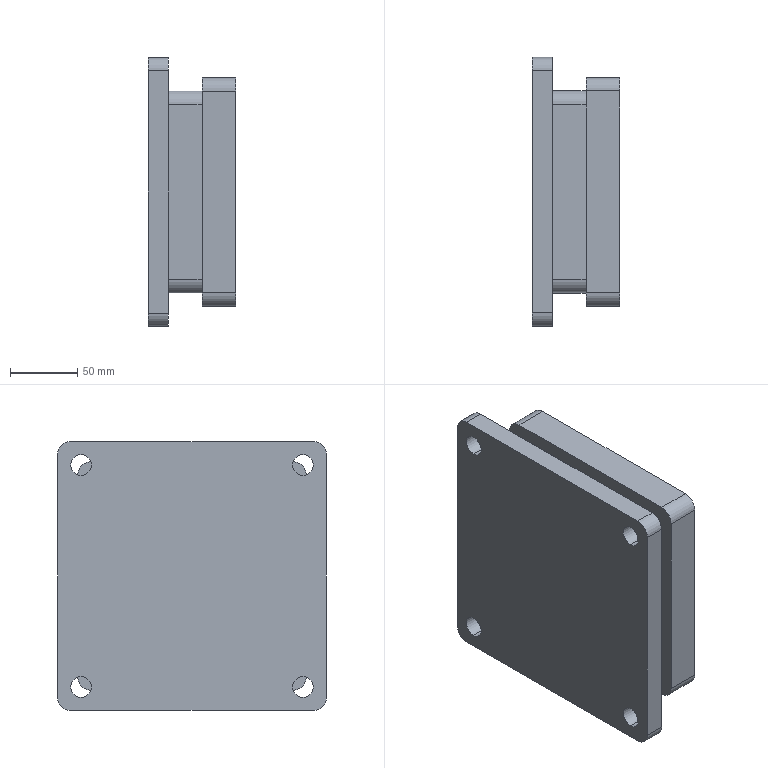Part | STEP file | part 322(default_machined_)-1.STEP | 2 solids | 46 faces | box 65 x 200 x 200 mm | volume 1280743 mm3 | cylinder 24 | plane 22 | commonest cylinder face diameters 20 x12 15.5 x8 10 x4
STEP:
#1=CARTESIAN_POINT('',(30.,-75.,85.));
#2=VERTEX_POINT('',#1);
#3=CARTESIAN_POINT('',(5.,-75.,85.));
#4=VERTEX_POINT('',#3);
#5=CARTESIAN_POINT('',(30.,-75.,85.));
#6=DIRECTION('',(-1.,0.,0.));
#7=VECTOR('',#6,1000.);
#8=LINE('',#5,#7);
#9=EDGE_CURVE('',#2,#4,#8,.T.);
#10=ORIENTED_EDGE('',*,*,#9,.T.);
#11=CARTESIAN_POINT('',(5.,-85.,75.));
#12=VERTEX_POINT('',#11);
#13=CARTESIAN_POINT('',(5.,-75.,75.));
#14=DIRECTION('',(1.,0.,0.));
#15=DIRECTION('',(0.,0.,-1.));
#16=AXIS2_PLACEMENT_3D('',#13,#14,#15);
#17=CIRCLE('',#16,10.);
#18=EDGE_CURVE('',#4,#12,#17,.T.);
#19=ORIENTED_EDGE('',*,*,#18,.T.);
#20=CARTESIAN_POINT('',(30.,-85.,75.));
#21=VERTEX_POINT('',#20);
#22=CARTESIAN_POINT('',(30.,-85.,75.));
#23=DIRECTION('',(-1.,0.,0.));
#24=VECTOR('',#23,1000.);
#25=LINE('',#22,#24);
#26=EDGE_CURVE('',#21,#12,#25,.T.);
#27=ORIENTED_EDGE('',*,*,#26,.F.);
#28=CARTESIAN_POINT('',(30.,-75.,75.));
#29=DIRECTION('',(1.,0.,0.));
#30=DIRECTION('',(0.,0.,-1.));
#31=AXIS2_PLACEMENT_3D('',#28,#29,#30);
#32=CIRCLE('',#31,10.);
#33=EDGE_CURVE('',#2,#21,#32,.T.);
#34=ORIENTED_EDGE('',*,*,#33,.F.);
#35=EDGE_LOOP('',(#10,#19,#27,#34));
#36=FACE_OUTER_BOUND('',#35,.T.);
#37=CARTESIAN_POINT('',(30.,-75.,75.));
#38=DIRECTION('',(-1.,0.,0.));
#39=DIRECTION('',(0.,0.,1.));
#40=AXIS2_PLACEMENT_3D('',#37,#38,#39);
#41=CYLINDRICAL_SURFACE('',#40,10.);
#42=ADVANCED_FACE('',(#36),#41,.T.);
#43=CARTESIAN_POINT('',(30.,75.,85.));
#44=VERTEX_POINT('',#43);
#45=CARTESIAN_POINT('',(5.,75.,85.));
#46=VERTEX_POINT('',#45);
#47=CARTESIAN_POINT('',(30.,75.,85.));
#48=DIRECTION('',(-1.,0.,0.));
#49=VECTOR('',#48,1000.);
#50=LINE('',#47,#49);
#51=EDGE_CURVE('',#44,#46,#50,.T.);
#52=ORIENTED_EDGE('',*,*,#51,.T.);
#53=CARTESIAN_POINT('',(5.,75.,85.));
#54=DIRECTION('',(0.,-1.,0.));
#55=VECTOR('',#54,1000.);
#56=LINE('',#53,#55);
#57=EDGE_CURVE('',#46,#4,#56,.T.);
#58=ORIENTED_EDGE('',*,*,#57,.T.);
#59=ORIENTED_EDGE('',*,*,#9,.F.);
#60=CARTESIAN_POINT('',(30.,75.,85.));
#61=DIRECTION('',(0.,-1.,0.));
#62=VECTOR('',#61,1000.);
#63=LINE('',#60,#62);
#64=EDGE_CURVE('',#44,#2,#63,.T.);
#65=ORIENTED_EDGE('',*,*,#64,.F.);
#66=EDGE_LOOP('',(#52,#58,#59,#65));
#67=FACE_OUTER_BOUND('',#66,.T.);
#68=CARTESIAN_POINT('',(30.,75.,85.));
#69=DIRECTION('',(0.,0.,-1.));
#70=DIRECTION('',(-1.,0.,0.));
#71=AXIS2_PLACEMENT_3D('',#68,#69,#70);
#72=PLANE('',#71);
#73=ADVANCED_FACE('',(#67),#72,.F.);
#74=CARTESIAN_POINT('',(30.,85.,75.));
#75=VERTEX_POINT('',#74);
#76=CARTESIAN_POINT('',(5.,85.,75.));
#77=VERTEX_POINT('',#76);
#78=CARTESIAN_POINT('',(30.,85.,75.));
#79=DIRECTION('',(-1.,0.,0.));
#80=VECTOR('',#79,1000.);
#81=LINE('',#78,#80);
#82=EDGE_CURVE('',#75,#77,#81,.T.);
#83=ORIENTED_EDGE('',*,*,#82,.T.);
#84=CARTESIAN_POINT('',(5.,75.,75.));
#85=DIRECTION('',(1.,0.,0.));
#86=DIRECTION('',(0.,0.,-1.));
#87=AXIS2_PLACEMENT_3D('',#84,#85,#86);
#88=CIRCLE('',#87,10.);
#89=EDGE_CURVE('',#77,#46,#88,.T.);
#90=ORIENTED_EDGE('',*,*,#89,.T.);
#91=ORIENTED_EDGE('',*,*,#51,.F.);
#92=CARTESIAN_POINT('',(30.,75.,75.));
#93=DIRECTION('',(1.,0.,0.));
#94=DIRECTION('',(0.,0.,-1.));
#95=AXIS2_PLACEMENT_3D('',#92,#93,#94);
#96=CIRCLE('',#95,10.);
#97=EDGE_CURVE('',#75,#44,#96,.T.);
#98=ORIENTED_EDGE('',*,*,#97,.F.);
#99=EDGE_LOOP('',(#83,#90,#91,#98));
#100=FACE_OUTER_BOUND('',#99,.T.);
#101=CARTESIAN_POINT('',(30.,75.,75.));
#102=DIRECTION('',(-1.,0.,0.));
#103=DIRECTION('',(0.,0.,1.));
#104=AXIS2_PLACEMENT_3D('',#101,#102,#103);
#105=CYLINDRICAL_SURFACE('',#104,10.);
#106=ADVANCED_FACE('',(#100),#105,.T.);
#107=CARTESIAN_POINT('',(30.,85.,-75.));
#108=VERTEX_POINT('',#107);
#109=CARTESIAN_POINT('',(5.,85.,-75.));
#110=VERTEX_POINT('',#109);
#111=CARTESIAN_POINT('',(30.,85.,-75.));
#112=DIRECTION('',(-1.,0.,0.));
#113=VECTOR('',#112,1000.);
#114=LINE('',#111,#113);
#115=EDGE_CURVE('',#108,#110,#114,.T.);
#116=ORIENTED_EDGE('',*,*,#115,.T.);
#117=CARTESIAN_POINT('',(5.,85.,75.));
#118=DIRECTION('',(0.,0.,1.));
#119=VECTOR('',#118,1000.);
#120=LINE('',#117,#119);
#121=EDGE_CURVE('',#110,#77,#120,.T.);
#122=ORIENTED_EDGE('',*,*,#121,.T.);
#123=ORIENTED_EDGE('',*,*,#82,.F.);
#124=CARTESIAN_POINT('',(30.,85.,-75.));
#125=DIRECTION('',(0.,0.,1.));
#126=VECTOR('',#125,1000.);
#127=LINE('',#124,#126);
#128=EDGE_CURVE('',#108,#75,#127,.T.);
#129=ORIENTED_EDGE('',*,*,#128,.F.);
#130=EDGE_LOOP('',(#116,#122,#123,#129));
#131=FACE_OUTER_BOUND('',#130,.T.);
#132=CARTESIAN_POINT('',(30.,85.,-75.));
#133=DIRECTION('',(0.,-1.,0.));
#134=DIRECTION('',(0.,0.,-1.));
#135=AXIS2_PLACEMENT_3D('',#132,#133,#134);
#136=PLANE('',#135);
#137=ADVANCED_FACE('',(#131),#136,.F.);
#138=CARTESIAN_POINT('',(30.,75.,-85.));
#139=VERTEX_POINT('',#138);
#140=CARTESIAN_POINT('',(5.,75.,-85.));
#141=VERTEX_POINT('',#140);
#142=CARTESIAN_POINT('',(30.,75.,-85.));
#143=DIRECTION('',(-1.,0.,0.));
#144=VECTOR('',#143,1000.);
#145=LINE('',#142,#144);
#146=EDGE_CURVE('',#139,#141,#145,.T.);
#147=ORIENTED_EDGE('',*,*,#146,.T.);
#148=CARTESIAN_POINT('',(5.,75.,-75.));
#149=DIRECTION('',(1.,0.,0.));
#150=DIRECTION('',(0.,0.,-1.));
#151=AXIS2_PLACEMENT_3D('',#148,#149,#150);
#152=CIRCLE('',#151,10.);
#153=EDGE_CURVE('',#141,#110,#152,.T.);
#154=ORIENTED_EDGE('',*,*,#153,.T.);
#155=ORIENTED_EDGE('',*,*,#115,.F.);
#156=CARTESIAN_POINT('',(30.,75.,-75.));
#157=DIRECTION('',(1.,0.,0.));
#158=DIRECTION('',(0.,0.,-1.));
#159=AXIS2_PLACEMENT_3D('',#156,#157,#158);
#160=CIRCLE('',#159,10.);
#161=EDGE_CURVE('',#139,#108,#160,.T.);
#162=ORIENTED_EDGE('',*,*,#161,.F.);
#163=EDGE_LOOP('',(#147,#154,#155,#162));
#164=FACE_OUTER_BOUND('',#163,.T.);
#165=CARTESIAN_POINT('',(30.,75.,-75.));
#166=DIRECTION('',(-1.,0.,0.));
#167=DIRECTION('',(0.,0.,1.));
#168=AXIS2_PLACEMENT_3D('',#165,#166,#167);
#169=CYLINDRICAL_SURFACE('',#168,10.);
#170=ADVANCED_FACE('',(#164),#169,.T.);
#171=CARTESIAN_POINT('',(30.,-75.,-85.));
#172=VERTEX_POINT('',#171);
#173=CARTESIAN_POINT('',(5.,-75.,-85.));
#174=VERTEX_POINT('',#173);
#175=CARTESIAN_POINT('',(30.,-75.,-85.));
#176=DIRECTION('',(-1.,0.,0.));
#177=VECTOR('',#176,1000.);
#178=LINE('',#175,#177);
#179=EDGE_CURVE('',#172,#174,#178,.T.);
#180=ORIENTED_EDGE('',*,*,#179,.T.);
#181=CARTESIAN_POINT('',(5.,75.,-85.));
#182=DIRECTION('',(0.,1.,0.));
#183=VECTOR('',#182,1000.);
#184=LINE('',#181,#183);
#185=EDGE_CURVE('',#174,#141,#184,.T.);
#186=ORIENTED_EDGE('',*,*,#185,.T.);
#187=ORIENTED_EDGE('',*,*,#146,.F.);
#188=CARTESIAN_POINT('',(30.,-75.,-85.));
#189=DIRECTION('',(0.,1.,0.));
#190=VECTOR('',#189,1000.);
#191=LINE('',#188,#190);
#192=EDGE_CURVE('',#172,#139,#191,.T.);
#193=ORIENTED_EDGE('',*,*,#192,.F.);
#194=EDGE_LOOP('',(#180,#186,#187,#193));
#195=FACE_OUTER_BOUND('',#194,.T.);
#196=CARTESIAN_POINT('',(30.,-75.,-85.));
#197=DIRECTION('',(0.,0.,1.));
#198=DIRECTION('',(0.,-1.,0.));
#199=AXIS2_PLACEMENT_3D('',#196,#197,#198);
#200=PLANE('',#199);
#201=ADVANCED_FACE('',(#195),#200,.F.);
#202=CARTESIAN_POINT('',(30.,-85.,-75.));
#203=VERTEX_POINT('',#202);
#204=CARTESIAN_POINT('',(5.,-85.,-75.));
#205=VERTEX_POINT('',#204);
#206=CARTESIAN_POINT('',(30.,-85.,-75.));
#207=DIRECTION('',(-1.,0.,0.));
#208=VECTOR('',#207,1000.);
#209=LINE('',#206,#208);
#210=EDGE_CURVE('',#203,#205,#209,.T.);
#211=ORIENTED_EDGE('',*,*,#210,.T.);
#212=CARTESIAN_POINT('',(5.,-75.,-75.));
#213=DIRECTION('',(1.,0.,0.));
#214=DIRECTION('',(0.,0.,-1.));
#215=AXIS2_PLACEMENT_3D('',#212,#213,#214);
#216=CIRCLE('',#215,10.);
#217=EDGE_CURVE('',#205,#174,#216,.T.);
#218=ORIENTED_EDGE('',*,*,#217,.T.);
#219=ORIENTED_EDGE('',*,*,#179,.F.);
#220=CARTESIAN_POINT('',(30.,-75.,-75.));
#221=DIRECTION('',(1.,0.,0.));
#222=DIRECTION('',(0.,0.,-1.));
#223=AXIS2_PLACEMENT_3D('',#220,#221,#222);
#224=CIRCLE('',#223,10.);
#225=EDGE_CURVE('',#203,#172,#224,.T.);
#226=ORIENTED_EDGE('',*,*,#225,.F.);
#227=EDGE_LOOP('',(#211,#218,#219,#226));
#228=FACE_OUTER_BOUND('',#227,.T.);
#229=CARTESIAN_POINT('',(30.,-75.,-75.));
#230=DIRECTION('',(-1.,0.,0.));
#231=DIRECTION('',(0.,0.,1.));
#232=AXIS2_PLACEMENT_3D('',#229,#230,#231);
#233=CYLINDRICAL_SURFACE('',#232,10.);
#234=ADVANCED_FACE('',(#228),#233,.T.);
#235=ORIENTED_EDGE('',*,*,#26,.T.);
#236=CARTESIAN_POINT('',(5.,-85.,75.));
#237=DIRECTION('',(0.,0.,-1.));
#238=VECTOR('',#237,1000.);
#239=LINE('',#236,#238);
#240=EDGE_CURVE('',#12,#205,#239,.T.);
#241=ORIENTED_EDGE('',*,*,#240,.T.);
#242=ORIENTED_EDGE('',*,*,#210,.F.);
#243=CARTESIAN_POINT('',(30.,-85.,75.));
#244=DIRECTION('',(0.,0.,-1.));
#245=VECTOR('',#244,1000.);
#246=LINE('',#243,#245);
#247=EDGE_CURVE('',#21,#203,#246,.T.);
#248=ORIENTED_EDGE('',*,*,#247,.F.);
#249=EDGE_LOOP('',(#235,#241,#242,#248));
#250=FACE_OUTER_BOUND('',#249,.T.);
#251=CARTESIAN_POINT('',(30.,-85.,75.));
#252=DIRECTION('',(0.,1.,0.));
#253=DIRECTION('',(0.,0.,-1.));
#254=AXIS2_PLACEMENT_3D('',#251,#252,#253);
#255=PLANE('',#254);
#256=ADVANCED_FACE('',(#250),#255,.F.);
#257=ORIENTED_EDGE('',*,*,#33,.T.);
#258=ORIENTED_EDGE('',*,*,#247,.T.);
#259=ORIENTED_EDGE('',*,*,#225,.T.);
#260=ORIENTED_EDGE('',*,*,#192,.T.);
#261=ORIENTED_EDGE('',*,*,#161,.T.);
#262=ORIENTED_EDGE('',*,*,#128,.T.);
#263=ORIENTED_EDGE('',*,*,#97,.T.);
#264=ORIENTED_EDGE('',*,*,#64,.T.);
#265=EDGE_LOOP('',(#257,#258,#259,#260,#261,#262,#263,#264));
#266=FACE_OUTER_BOUND('',#265,.T.);
#267=CARTESIAN_POINT('',(30.,-75.,75.));
#268=DIRECTION('',(1.,0.,0.));
#269=DIRECTION('',(0.,1.,0.));
#270=AXIS2_PLACEMENT_3D('',#267,#268,#269);
#271=PLANE('',#270);
#272=ADVANCED_FACE('',(#266),#271,.T.);
#273=CARTESIAN_POINT('',(5.,75.,-65.));
#274=VERTEX_POINT('',#273);
#275=CARTESIAN_POINT('',(5.,75.,65.));
#276=VERTEX_POINT('',#275);
#277=CARTESIAN_POINT('',(5.,75.,-65.));
#278=DIRECTION('',(0.,0.,1.));
#279=VECTOR('',#278,1000.);
#280=LINE('',#277,#279);
#281=EDGE_CURVE('',#274,#276,#280,.T.);
#282=ORIENTED_EDGE('',*,*,#281,.T.);
#283=CARTESIAN_POINT('',(5.,65.,75.));
#284=VERTEX_POINT('',#283);
#285=CARTESIAN_POINT('',(5.,65.,65.));
#286=DIRECTION('',(1.,0.,0.));
#287=DIRECTION('',(0.,0.,-1.));
#288=AXIS2_PLACEMENT_3D('',#285,#286,#287);
#289=CIRCLE('',#288,10.);
#290=EDGE_CURVE('',#276,#284,#289,.T.);
#291=ORIENTED_EDGE('',*,*,#290,.T.);
#292=CARTESIAN_POINT('',(5.,-65.,75.));
#293=VERTEX_POINT('',#292);
#294=CARTESIAN_POINT('',(5.,65.,75.));
#295=DIRECTION('',(0.,-1.,0.));
#296=VECTOR('',#295,1000.);
#297=LINE('',#294,#296);
#298=EDGE_CURVE('',#284,#293,#297,.T.);
#299=ORIENTED_EDGE('',*,*,#298,.T.);
#300=CARTESIAN_POINT('',(5.,-75.,65.));
#301=VERTEX_POINT('',#300);
#302=CARTESIAN_POINT('',(5.,-65.,65.));
#303=DIRECTION('',(1.,0.,0.));
#304=DIRECTION('',(0.,0.,-1.));
#305=AXIS2_PLACEMENT_3D('',#302,#303,#304);
#306=CIRCLE('',#305,10.);
#307=EDGE_CURVE('',#293,#301,#306,.T.);
#308=ORIENTED_EDGE('',*,*,#307,.T.);
#309=CARTESIAN_POINT('',(5.,-75.,-65.));
#310=VERTEX_POINT('',#309);
#311=CARTESIAN_POINT('',(5.,-75.,65.));
#312=DIRECTION('',(0.,0.,-1.));
#313=VECTOR('',#312,1000.);
#314=LINE('',#311,#313);
#315=EDGE_CURVE('',#301,#310,#314,.T.);
#316=ORIENTED_EDGE('',*,*,#315,.T.);
#317=CARTESIAN_POINT('',(5.,-65.,-75.));
#318=VERTEX_POINT('',#317);
#319=CARTESIAN_POINT('',(5.,-65.,-65.));
#320=DIRECTION('',(1.,0.,0.));
#321=DIRECTION('',(0.,0.,-1.));
#322=AXIS2_PLACEMENT_3D('',#319,#320,#321);
#323=CIRCLE('',#322,10.);
#324=EDGE_CURVE('',#310,#318,#323,.T.);
#325=ORIENTED_EDGE('',*,*,#324,.T.);
#326=CARTESIAN_POINT('',(5.,65.,-75.));
#327=VERTEX_POINT('',#326);
#328=CARTESIAN_POINT('',(5.,-65.,-75.));
#329=DIRECTION('',(0.,1.,0.));
#330=VECTOR('',#329,1000.);
#331=LINE('',#328,#330);
#332=EDGE_CURVE('',#318,#327,#331,.T.);
#333=ORIENTED_EDGE('',*,*,#332,.T.);
#334=CARTESIAN_POINT('',(5.,65.,-65.));
#335=DIRECTION('',(1.,0.,0.));
#336=DIRECTION('',(0.,0.,-1.));
#337=AXIS2_PLACEMENT_3D('',#334,#335,#336);
#338=CIRCLE('',#337,10.);
#339=EDGE_CURVE('',#327,#274,#338,.T.);
#340=ORIENTED_EDGE('',*,*,#339,.T.);
#341=EDGE_LOOP('',(#282,#291,#299,#308,#316,#325,#333,#340));
#342=FACE_BOUND('',#341,.T.);
#343=ORIENTED_EDGE('',*,*,#18,.F.);
#344=ORIENTED_EDGE('',*,*,#57,.F.);
#345=ORIENTED_EDGE('',*,*,#89,.F.);
#346=ORIENTED_EDGE('',*,*,#121,.F.);
#347=ORIENTED_EDGE('',*,*,#153,.F.);
#348=ORIENTED_EDGE('',*,*,#185,.F.);
#349=ORIENTED_EDGE('',*,*,#217,.F.);
#350=ORIENTED_EDGE('',*,*,#240,.F.);
#351=EDGE_LOOP('',(#343,#344,#345,#346,#347,#348,#349,#350));
#352=FACE_OUTER_BOUND('',#351,.T.);
#353=CARTESIAN_POINT('',(5.,-75.,75.));
#354=DIRECTION('',(1.,0.,0.));
#355=DIRECTION('',(0.,1.,0.));
#356=AXIS2_PLACEMENT_3D('',#353,#354,#355);
#357=PLANE('',#356);
#358=ADVANCED_FACE('',(#342,#352),#357,.F.);
#359=CARTESIAN_POINT('',(10.,65.,-70.));
#360=VERTEX_POINT('',#359);
#361=CARTESIAN_POINT('',(10.,70.,-65.));
#362=VERTEX_POINT('',#361);
#363=CARTESIAN_POINT('',(10.,65.,-65.));
#364=DIRECTION('',(1.,0.,0.));
#365=DIRECTION('',(0.,0.,-1.));
#366=AXIS2_PLACEMENT_3D('',#363,#364,#365);
#367=CIRCLE('',#366,5.);
#368=EDGE_CURVE('',#360,#362,#367,.T.);
#369=ORIENTED_EDGE('',*,*,#368,.F.);
#370=CARTESIAN_POINT('',(10.,-65.,-70.));
#371=VERTEX_POINT('',#370);
#372=CARTESIAN_POINT('',(10.,-65.,-70.));
#373=DIRECTION('',(0.,1.,0.));
#374=VECTOR('',#373,1000.);
#375=LINE('',#372,#374);
#376=EDGE_CURVE('',#371,#360,#375,.T.);
#377=ORIENTED_EDGE('',*,*,#376,.F.);
#378=CARTESIAN_POINT('',(10.,-70.,-65.));
#379=VERTEX_POINT('',#378);
#380=CARTESIAN_POINT('',(10.,-65.,-65.));
#381=DIRECTION('',(1.,0.,0.));
#382=DIRECTION('',(0.,0.,-1.));
#383=AXIS2_PLACEMENT_3D('',#380,#381,#382);
#384=CIRCLE('',#383,5.);
#385=EDGE_CURVE('',#379,#371,#384,.T.);
#386=ORIENTED_EDGE('',*,*,#385,.F.);
#387=CARTESIAN_POINT('',(10.,-70.,65.));
#388=VERTEX_POINT('',#387);
#389=CARTESIAN_POINT('',(10.,-70.,65.));
#390=DIRECTION('',(0.,0.,-1.));
#391=VECTOR('',#390,1000.);
#392=LINE('',#389,#391);
#393=EDGE_CURVE('',#388,#379,#392,.T.);
#394=ORIENTED_EDGE('',*,*,#393,.F.);
#395=CARTESIAN_POINT('',(10.,-65.,70.));
#396=VERTEX_POINT('',#395);
#397=CARTESIAN_POINT('',(10.,-65.,65.));
#398=DIRECTION('',(1.,0.,0.));
#399=DIRECTION('',(0.,0.,-1.));
#400=AXIS2_PLACEMENT_3D('',#397,#398,#399);
#401=CIRCLE('',#400,5.);
#402=EDGE_CURVE('',#396,#388,#401,.T.);
#403=ORIENTED_EDGE('',*,*,#402,.F.);
#404=CARTESIAN_POINT('',(10.,65.,70.));
#405=VERTEX_POINT('',#404);
#406=CARTESIAN_POINT('',(10.,65.,70.));
#407=DIRECTION('',(0.,-1.,0.));
#408=VECTOR('',#407,1000.);
#409=LINE('',#406,#408);
#410=EDGE_CURVE('',#405,#396,#409,.T.);
#411=ORIENTED_EDGE('',*,*,#410,.F.);
#412=CARTESIAN_POINT('',(10.,70.,65.));
#413=VERTEX_POINT('',#412);
#414=CARTESIAN_POINT('',(10.,65.,65.));
#415=DIRECTION('',(1.,0.,0.));
#416=DIRECTION('',(0.,0.,-1.));
#417=AXIS2_PLACEMENT_3D('',#414,#415,#416);
#418=CIRCLE('',#417,5.);
#419=EDGE_CURVE('',#413,#405,#418,.T.);
#420=ORIENTED_EDGE('',*,*,#419,.F.);
#421=CARTESIAN_POINT('',(10.,70.,-65.));
#422=DIRECTION('',(0.,0.,1.));
#423=VECTOR('',#422,1000.);
#424=LINE('',#421,#423);
#425=EDGE_CURVE('',#362,#413,#424,.T.);
#426=ORIENTED_EDGE('',*,*,#425,.F.);
#427=EDGE_LOOP('',(#369,#377,#386,#394,#403,#411,#420,#426));
#428=FACE_OUTER_BOUND('',#427,.T.);
#429=CARTESIAN_POINT('',(10.,65.,-65.));
#430=DIRECTION('',(1.,0.,0.));
#431=DIRECTION('',(0.,1.,0.));
#432=AXIS2_PLACEMENT_3D('',#429,#430,#431);
#433=PLANE('',#432);
#434=ADVANCED_FACE('',(#428),#433,.F.);
#435=CARTESIAN_POINT('',(-20.,-65.,70.));
#436=VERTEX_POINT('',#435);
#437=CARTESIAN_POINT('',(-20.,-70.,65.));
#438=VERTEX_POINT('',#437);
#439=CARTESIAN_POINT('',(-20.,-65.,65.));
#440=DIRECTION('',(1.,0.,0.));
#441=DIRECTION('',(0.,1.,0.));
#442=AXIS2_PLACEMENT_3D('',#439,#440,#441);
#443=CIRCLE('',#442,5.);
#444=EDGE_CURVE('',#436,#438,#443,.T.);
#445=ORIENTED_EDGE('',*,*,#444,.T.);
#446=CARTESIAN_POINT('',(-20.,-70.,-65.));
#447=VERTEX_POINT('',#446);
#448=CARTESIAN_POINT('',(-20.,-70.,-65.));
#449=DIRECTION('',(0.,0.,-1.));
#450=VECTOR('',#449,1000.);
#451=LINE('',#448,#450);
#452=EDGE_CURVE('',#438,#447,#451,.T.);
#453=ORIENTED_EDGE('',*,*,#452,.T.);
#454=CARTESIAN_POINT('',(-20.,-65.,-70.));
#455=VERTEX_POINT('',#454);
#456=CARTESIAN_POINT('',(-20.,-65.,-65.));
#457=DIRECTION('',(1.,0.,0.));
#458=DIRECTION('',(0.,1.,0.));
#459=AXIS2_PLACEMENT_3D('',#456,#457,#458);
#460=CIRCLE('',#459,5.);
#461=EDGE_CURVE('',#447,#455,#460,.T.);
#462=ORIENTED_EDGE('',*,*,#461,.T.);
#463=CARTESIAN_POINT('',(-20.,65.,-70.));
#464=VERTEX_POINT('',#463);
#465=CARTESIAN_POINT('',(-20.,-65.,-70.));
#466=DIRECTION('',(0.,1.,0.));
#467=VECTOR('',#466,1000.);
#468=LINE('',#465,#467);
#469=EDGE_CURVE('',#455,#464,#468,.T.);
#470=ORIENTED_EDGE('',*,*,#469,.T.);
#471=CARTESIAN_POINT('',(-20.,70.,-65.));
#472=VERTEX_POINT('',#471);
#473=CARTESIAN_POINT('',(-20.,65.,-65.));
#474=DIRECTION('',(1.,0.,0.));
#475=DIRECTION('',(0.,1.,0.));
#476=AXIS2_PLACEMENT_3D('',#473,#474,#475);
#477=CIRCLE('',#476,5.);
#478=EDGE_CURVE('',#464,#472,#477,.T.);
#479=ORIENTED_EDGE('',*,*,#478,.T.);
#480=CARTESIAN_POINT('',(-20.,70.,65.));
#481=VERTEX_POINT('',#480);
#482=CARTESIAN_POINT('',(-20.,70.,65.));
#483=DIRECTION('',(0.,0.,1.));
#484=VECTOR('',#483,1000.);
#485=LINE('',#482,#484);
#486=EDGE_CURVE('',#472,#481,#485,.T.);
#487=ORIENTED_EDGE('',*,*,#486,.T.);
#488=CARTESIAN_POINT('',(-20.,65.,70.));
#489=VERTEX_POINT('',#488);
#490=CARTESIAN_POINT('',(-20.,65.,65.));
#491=DIRECTION('',(1.,0.,0.));
#492=DIRECTION('',(0.,1.,0.));
#493=AXIS2_PLACEMENT_3D('',#490,#491,#492);
#494=CIRCLE('',#493,5.);
#495=EDGE_CURVE('',#481,#489,#494,.T.);
#496=ORIENTED_EDGE('',*,*,#495,.T.);
#497=CARTESIAN_POINT('',(-20.,65.,70.));
#498=DIRECTION('',(0.,-1.,0.));
#499=VECTOR('',#498,1000.);
#500=LINE('',#497,#499);
#501=EDGE_CURVE('',#489,#436,#500,.T.);
#502=ORIENTED_EDGE('',*,*,#501,.T.);
#503=EDGE_LOOP('',(#445,#453,#462,#470,#479,#487,#496,#502));
#504=FACE_BOUND('',#503,.T.);
#505=CARTESIAN_POINT('',(-20.,75.,65.));
#506=VERTEX_POINT('',#505);
#507=CARTESIAN_POINT('',(-20.,65.,75.));
#508=VERTEX_POINT('',#507);
#509=CARTESIAN_POINT('',(-20.,65.,65.));
#510=DIRECTION('',(1.,0.,0.));
#511=DIRECTION('',(0.,1.,0.));
#512=AXIS2_PLACEMENT_3D('',#509,#510,#511);
#513=CIRCLE('',#512,10.);
#514=EDGE_CURVE('',#506,#508,#513,.T.);
#515=ORIENTED_EDGE('',*,*,#514,.F.);
#516=CARTESIAN_POINT('',(-20.,75.,-65.));
#517=VERTEX_POINT('',#516);
#518=CARTESIAN_POINT('',(-20.,75.,65.));
#519=DIRECTION('',(0.,0.,1.));
#520=VECTOR('',#519,1000.);
#521=LINE('',#518,#520);
#522=EDGE_CURVE('',#517,#506,#521,.T.);
#523=ORIENTED_EDGE('',*,*,#522,.F.);
#524=CARTESIAN_POINT('',(-20.,65.,-75.));
#525=VERTEX_POINT('',#524);
#526=CARTESIAN_POINT('',(-20.,65.,-65.));
#527=DIRECTION('',(1.,0.,0.));
#528=DIRECTION('',(0.,1.,0.));
#529=AXIS2_PLACEMENT_3D('',#526,#527,#528);
#530=CIRCLE('',#529,10.);
#531=EDGE_CURVE('',#525,#517,#530,.T.);
#532=ORIENTED_EDGE('',*,*,#531,.F.);
#533=CARTESIAN_POINT('',(-20.,-65.,-75.));
#534=VERTEX_POINT('',#533);
#535=CARTESIAN_POINT('',(-20.,-65.,-75.));
#536=DIRECTION('',(0.,1.,0.));
#537=VECTOR('',#536,1000.);
#538=LINE('',#535,#537);
#539=EDGE_CURVE('',#534,#525,#538,.T.);
#540=ORIENTED_EDGE('',*,*,#539,.F.);
#541=CARTESIAN_POINT('',(-20.,-75.,-65.));
#542=VERTEX_POINT('',#541);
#543=CARTESIAN_POINT('',(-20.,-65.,-65.));
#544=DIRECTION('',(1.,0.,0.));
#545=DIRECTION('',(0.,1.,0.));
#546=AXIS2_PLACEMENT_3D('',#543,#544,#545);
#547=CIRCLE('',#546,10.);
#548=EDGE_CURVE('',#542,#534,#547,.T.);
#549=ORIENTED_EDGE('',*,*,#548,.F.);
#550=CARTESIAN_POINT('',(-20.,-75.,65.));
#551=VERTEX_POINT('',#550);
#552=CARTESIAN_POINT('',(-20.,-75.,-65.));
#553=DIRECTION('',(0.,0.,-1.));
#554=VECTOR('',#553,1000.);
#555=LINE('',#552,#554);
#556=EDGE_CURVE('',#551,#542,#555,.T.);
#557=ORIENTED_EDGE('',*,*,#556,.F.);
#558=CARTESIAN_POINT('',(-20.,-65.,75.));
#559=VERTEX_POINT('',#558);
#560=CARTESIAN_POINT('',(-20.,-65.,65.));
#561=DIRECTION('',(1.,0.,0.));
#562=DIRECTION('',(0.,1.,0.));
#563=AXIS2_PLACEMENT_3D('',#560,#561,#562);
#564=CIRCLE('',#563,10.);
#565=EDGE_CURVE('',#559,#551,#564,.T.);
#566=ORIENTED_EDGE('',*,*,#565,.F.);
#567=CARTESIAN_POINT('',(-20.,65.,75.));
#568=DIRECTION('',(0.,-1.,0.));
#569=VECTOR('',#568,1000.);
#570=LINE('',#567,#569);
#571=EDGE_CURVE('',#508,#559,#570,.T.);
#572=ORIENTED_EDGE('',*,*,#571,.F.);
#573=EDGE_LOOP('',(#515,#523,#532,#540,#549,#557,#566,#572));
#574=FACE_OUTER_BOUND('',#573,.T.);
#575=CARTESIAN_POINT('',(-20.,65.,65.));
#576=DIRECTION('',(1.,0.,0.));
#577=DIRECTION('',(0.,1.,0.));
#578=AXIS2_PLACEMENT_3D('',#575,#576,#577);
#579=PLANE('',#578);
#580=ADVANCED_FACE('',(#504,#574),#579,.F.);
#581=CARTESIAN_POINT('',(20.,-70.,65.));
#582=DIRECTION('',(-1.,0.,0.));
#583=VECTOR('',#582,1000.);
#584=LINE('',#581,#583);
#585=EDGE_CURVE('',#388,#438,#584,.T.);
#586=ORIENTED_EDGE('',*,*,#585,.F.);
#587=ORIENTED_EDGE('',*,*,#393,.T.);
#588=CARTESIAN_POINT('',(20.,-70.,-65.));
#589=DIRECTION('',(-1.,0.,0.));
#590=VECTOR('',#589,1000.);
#591=LINE('',#588,#590);
#592=EDGE_CURVE('',#379,#447,#591,.T.);
#593=ORIENTED_EDGE('',*,*,#592,.T.);
#594=ORIENTED_EDGE('',*,*,#452,.F.);
#595=EDGE_LOOP('',(#586,#587,#593,#594));
#596=FACE_OUTER_BOUND('',#595,.T.);
#597=CARTESIAN_POINT('',(20.,-70.,-65.));
#598=DIRECTION('',(0.,1.,0.));
#599=DIRECTION('',(0.,0.,-1.));
#600=AXIS2_PLACEMENT_3D('',#597,#598,#599);
#601=PLANE('',#600);
#602=ADVANCED_FACE('',(#596),#601,.T.);
#603=ORIENTED_EDGE('',*,*,#592,.F.);
#604=ORIENTED_EDGE('',*,*,#385,.T.);
#605=CARTESIAN_POINT('',(20.,-65.,-70.));
#606=DIRECTION('',(-1.,0.,0.));
#607=VECTOR('',#606,1000.);
#608=LINE('',#605,#607);
#609=EDGE_CURVE('',#371,#455,#608,.T.);
#610=ORIENTED_EDGE('',*,*,#609,.T.);
#611=ORIENTED_EDGE('',*,*,#461,.F.);
#612=EDGE_LOOP('',(#603,#604,#610,#611));
#613=FACE_OUTER_BOUND('',#612,.T.);
#614=CARTESIAN_POINT('',(20.,-65.,-65.));
#615=DIRECTION('',(-1.,0.,0.));
#616=DIRECTION('',(0.,-1.,0.));
#617=AXIS2_PLACEMENT_3D('',#614,#615,#616);
#618=CYLINDRICAL_SURFACE('',#617,5.);
#619=ADVANCED_FACE('',(#613),#618,.F.);
#620=ORIENTED_EDGE('',*,*,#609,.F.);
#621=ORIENTED_EDGE('',*,*,#376,.T.);
#622=CARTESIAN_POINT('',(20.,65.,-70.));
#623=DIRECTION('',(-1.,0.,0.));
#624=VECTOR('',#623,1000.);
#625=LINE('',#622,#624);
#626=EDGE_CURVE('',#360,#464,#625,.T.);
#627=ORIENTED_EDGE('',*,*,#626,.T.);
#628=ORIENTED_EDGE('',*,*,#469,.F.);
#629=EDGE_LOOP('',(#620,#621,#627,#628));
#630=FACE_OUTER_BOUND('',#629,.T.);
#631=CARTESIAN_POINT('',(20.,-65.,-70.));
#632=DIRECTION('',(0.,0.,1.));
#633=DIRECTION('',(0.,-1.,0.));
#634=AXIS2_PLACEMENT_3D('',#631,#632,#633);
#635=PLANE('',#634);
#636=ADVANCED_FACE('',(#630),#635,.T.);
#637=ORIENTED_EDGE('',*,*,#626,.F.);
#638=ORIENTED_EDGE('',*,*,#368,.T.);
#639=CARTESIAN_POINT('',(20.,70.,-65.));
#640=DIRECTION('',(-1.,0.,0.));
#641=VECTOR('',#640,1000.);
#642=LINE('',#639,#641);
#643=EDGE_CURVE('',#362,#472,#642,.T.);
#644=ORIENTED_EDGE('',*,*,#643,.T.);
#645=ORIENTED_EDGE('',*,*,#478,.F.);
#646=EDGE_LOOP('',(#637,#638,#644,#645));
#647=FACE_OUTER_BOUND('',#646,.T.);
#648=CARTESIAN_POINT('',(20.,65.,-65.));
#649=DIRECTION('',(-1.,0.,0.));
#650=DIRECTION('',(0.,-1.,0.));
#651=AXIS2_PLACEMENT_3D('',#648,#649,#650);
#652=CYLINDRICAL_SURFACE('',#651,5.);
#653=ADVANCED_FACE('',(#647),#652,.F.);
#654=ORIENTED_EDGE('',*,*,#643,.F.);
#655=ORIENTED_EDGE('',*,*,#425,.T.);
#656=CARTESIAN_POINT('',(20.,70.,65.));
#657=DIRECTION('',(-1.,0.,0.));
#658=VECTOR('',#657,1000.);
#659=LINE('',#656,#658);
#660=EDGE_CURVE('',#413,#481,#659,.T.);
#661=ORIENTED_EDGE('',*,*,#660,.T.);
#662=ORIENTED_EDGE('',*,*,#486,.F.);
#663=EDGE_LOOP('',(#654,#655,#661,#662));
#664=FACE_OUTER_BOUND('',#663,.T.);
#665=CARTESIAN_POINT('',(20.,70.,65.));
#666=DIRECTION('',(0.,-1.,0.));
#667=DIRECTION('',(0.,0.,-1.));
#668=AXIS2_PLACEMENT_3D('',#665,#666,#667);
#669=PLANE('',#668);
#670=ADVANCED_FACE('',(#664),#669,.T.);
#671=ORIENTED_EDGE('',*,*,#660,.F.);
#672=ORIENTED_EDGE('',*,*,#419,.T.);
#673=CARTESIAN_POINT('',(20.,65.,70.));
#674=DIRECTION('',(-1.,0.,0.));
#675=VECTOR('',#674,1000.);
#676=LINE('',#673,#675);
#677=EDGE_CURVE('',#405,#489,#676,.T.);
#678=ORIENTED_EDGE('',*,*,#677,.T.);
#679=ORIENTED_EDGE('',*,*,#495,.F.);
#680=EDGE_LOOP('',(#671,#672,#678,#679));
#681=FACE_OUTER_BOUND('',#680,.T.);
#682=CARTESIAN_POINT('',(20.,65.,65.));
#683=DIRECTION('',(-1.,0.,0.));
#684=DIRECTION('',(0.,-1.,0.));
#685=AXIS2_PLACEMENT_3D('',#682,#683,#684);
#686=CYLINDRICAL_SURFACE('',#685,5.);
#687=ADVANCED_FACE('',(#681),#686,.F.);
#688=ORIENTED_EDGE('',*,*,#677,.F.);
#689=ORIENTED_EDGE('',*,*,#410,.T.);
#690=CARTESIAN_POINT('',(20.,-65.,70.));
#691=DIRECTION('',(-1.,0.,0.));
#692=VECTOR('',#691,1000.);
#693=LINE('',#690,#692);
#694=EDGE_CURVE('',#396,#436,#693,.T.);
#695=ORIENTED_EDGE('',*,*,#694,.T.);
#696=ORIENTED_EDGE('',*,*,#501,.F.);
#697=EDGE_LOOP('',(#688,#689,#695,#696));
#698=FACE_OUTER_BOUND('',#697,.T.);
#699=CARTESIAN_POINT('',(20.,65.,70.));
#700=DIRECTION('',(0.,0.,-1.));
#701=DIRECTION('',(-1.,0.,0.));
#702=AXIS2_PLACEMENT_3D('',#699,#700,#701);
#703=PLANE('',#702);
#704=ADVANCED_FACE('',(#698),#703,.T.);
#705=ORIENTED_EDGE('',*,*,#694,.F.);
#706=ORIENTED_EDGE('',*,*,#402,.T.);
#707=ORIENTED_EDGE('',*,*,#585,.T.);
#708=ORIENTED_EDGE('',*,*,#444,.F.);
#709=EDGE_LOOP('',(#705,#706,#707,#708));
#710=FACE_OUTER_BOUND('',#709,.T.);
#711=CARTESIAN_POINT('',(20.,-65.,65.));
#712=DIRECTION('',(-1.,0.,0.));
#713=DIRECTION('',(0.,-1.,0.));
#714=AXIS2_PLACEMENT_3D('',#711,#712,#713);
#715=CYLINDRICAL_SURFACE('',#714,5.);
#716=ADVANCED_FACE('',(#710),#715,.F.);
#717=ORIENTED_EDGE('',*,*,#281,.F.);
#718=CARTESIAN_POINT('',(20.,75.,-65.));
#719=DIRECTION('',(-1.,0.,0.));
#720=VECTOR('',#719,1000.);
#721=LINE('',#718,#720);
#722=EDGE_CURVE('',#274,#517,#721,.T.);
#723=ORIENTED_EDGE('',*,*,#722,.T.);
#724=ORIENTED_EDGE('',*,*,#522,.T.);
#725=CARTESIAN_POINT('',(20.,75.,65.));
#726=DIRECTION('',(-1.,0.,0.));
#727=VECTOR('',#726,1000.);
#728=LINE('',#725,#727);
#729=EDGE_CURVE('',#276,#506,#728,.T.);
#730=ORIENTED_EDGE('',*,*,#729,.F.);
#731=EDGE_LOOP('',(#717,#723,#724,#730));
#732=FACE_OUTER_BOUND('',#731,.T.);
#733=CARTESIAN_POINT('',(20.,75.,65.));
#734=DIRECTION('',(0.,-1.,0.));
#735=DIRECTION('',(0.,0.,-1.));
#736=AXIS2_PLACEMENT_3D('',#733,#734,#735);
#737=PLANE('',#736);
#738=ADVANCED_FACE('',(#732),#737,.F.);
#739=ORIENTED_EDGE('',*,*,#339,.F.);
#740=CARTESIAN_POINT('',(20.,65.,-75.));
#741=DIRECTION('',(-1.,0.,0.));
#742=VECTOR('',#741,1000.);
#743=LINE('',#740,#742);
#744=EDGE_CURVE('',#327,#525,#743,.T.);
#745=ORIENTED_EDGE('',*,*,#744,.T.);
#746=ORIENTED_EDGE('',*,*,#531,.T.);
#747=ORIENTED_EDGE('',*,*,#722,.F.);
#748=EDGE_LOOP('',(#739,#745,#746,#747));
#749=FACE_OUTER_BOUND('',#748,.T.);
#750=CARTESIAN_POINT('',(20.,65.,-65.));
#751=DIRECTION('',(-1.,0.,0.));
#752=DIRECTION('',(0.,-1.,0.));
#753=AXIS2_PLACEMENT_3D('',#750,#751,#752);
#754=CYLINDRICAL_SURFACE('',#753,10.);
#755=ADVANCED_FACE('',(#749),#754,.T.);
#756=ORIENTED_EDGE('',*,*,#332,.F.);
#757=CARTESIAN_POINT('',(20.,-65.,-75.));
#758=DIRECTION('',(-1.,0.,0.));
#759=VECTOR('',#758,1000.);
#760=LINE('',#757,#759);
#761=EDGE_CURVE('',#318,#534,#760,.T.);
#762=ORIENTED_EDGE('',*,*,#761,.T.);
#763=ORIENTED_EDGE('',*,*,#539,.T.);
#764=ORIENTED_EDGE('',*,*,#744,.F.);
#765=EDGE_LOOP('',(#756,#762,#763,#764));
#766=FACE_OUTER_BOUND('',#765,.T.);
#767=CARTESIAN_POINT('',(20.,-65.,-75.));
#768=DIRECTION('',(0.,0.,1.));
#769=DIRECTION('',(0.,-1.,0.));
#770=AXIS2_PLACEMENT_3D('',#767,#768,#769);
#771=PLANE('',#770);
#772=ADVANCED_FACE('',(#766),#771,.F.);
#773=ORIENTED_EDGE('',*,*,#324,.F.);
#774=CARTESIAN_POINT('',(20.,-75.,-65.));
#775=DIRECTION('',(-1.,0.,0.));
#776=VECTOR('',#775,1000.);
#777=LINE('',#774,#776);
#778=EDGE_CURVE('',#310,#542,#777,.T.);
#779=ORIENTED_EDGE('',*,*,#778,.T.);
#780=ORIENTED_EDGE('',*,*,#548,.T.);
#781=ORIENTED_EDGE('',*,*,#761,.F.);
#782=EDGE_LOOP('',(#773,#779,#780,#781));
#783=FACE_OUTER_BOUND('',#782,.T.);
#784=CARTESIAN_POINT('',(20.,-65.,-65.));
#785=DIRECTION('',(-1.,0.,0.));
#786=DIRECTION('',(0.,-1.,0.));
#787=AXIS2_PLACEMENT_3D('',#784,#785,#786);
#788=CYLINDRICAL_SURFACE('',#787,10.);
#789=ADVANCED_FACE('',(#783),#788,.T.);
#790=ORIENTED_EDGE('',*,*,#315,.F.);
#791=CARTESIAN_POINT('',(20.,-75.,65.));
#792=DIRECTION('',(-1.,0.,0.));
#793=VECTOR('',#792,1000.);
#794=LINE('',#791,#793);
#795=EDGE_CURVE('',#301,#551,#794,.T.);
#796=ORIENTED_EDGE('',*,*,#795,.T.);
#797=ORIENTED_EDGE('',*,*,#556,.T.);
#798=ORIENTED_EDGE('',*,*,#778,.F.);
#799=EDGE_LOOP('',(#790,#796,#797,#798));
#800=FACE_OUTER_BOUND('',#799,.T.);
#801=CARTESIAN_POINT('',(20.,-75.,-65.));
#802=DIRECTION('',(0.,1.,0.));
#803=DIRECTION('',(0.,0.,-1.));
#804=AXIS2_PLACEMENT_3D('',#801,#802,#803);
#805=PLANE('',#804);
#806=ADVANCED_FACE('',(#800),#805,.F.);
#807=ORIENTED_EDGE('',*,*,#307,.F.);
#808=CARTESIAN_POINT('',(20.,-65.,75.));
#809=DIRECTION('',(-1.,0.,0.));
#810=VECTOR('',#809,1000.);
#811=LINE('',#808,#810);
#812=EDGE_CURVE('',#293,#559,#811,.T.);
#813=ORIENTED_EDGE('',*,*,#812,.T.);
#814=ORIENTED_EDGE('',*,*,#565,.T.);
#815=ORIENTED_EDGE('',*,*,#795,.F.);
#816=EDGE_LOOP('',(#807,#813,#814,#815));
#817=FACE_OUTER_BOUND('',#816,.T.);
#818=CARTESIAN_POINT('',(20.,-65.,65.));
#819=DIRECTION('',(-1.,0.,0.));
#820=DIRECTION('',(0.,-1.,0.));
#821=AXIS2_PLACEMENT_3D('',#818,#819,#820);
#822=CYLINDRICAL_SURFACE('',#821,10.);
#823=ADVANCED_FACE('',(#817),#822,.T.);
#824=ORIENTED_EDGE('',*,*,#298,.F.);
#825=CARTESIAN_POINT('',(20.,65.,75.));
#826=DIRECTION('',(-1.,0.,0.));
#827=VECTOR('',#826,1000.);
#828=LINE('',#825,#827);
#829=EDGE_CURVE('',#284,#508,#828,.T.);
#830=ORIENTED_EDGE('',*,*,#829,.T.);
#831=ORIENTED_EDGE('',*,*,#571,.T.);
#832=ORIENTED_EDGE('',*,*,#812,.F.);
#833=EDGE_LOOP('',(#824,#830,#831,#832));
#834=FACE_OUTER_BOUND('',#833,.T.);
#835=CARTESIAN_POINT('',(20.,65.,75.));
#836=DIRECTION('',(0.,0.,-1.));
#837=DIRECTION('',(-1.,0.,0.));
#838=AXIS2_PLACEMENT_3D('',#835,#836,#837);
#839=PLANE('',#838);
#840=ADVANCED_FACE('',(#834),#839,.F.);
#841=ORIENTED_EDGE('',*,*,#290,.F.);
#842=ORIENTED_EDGE('',*,*,#729,.T.);
#843=ORIENTED_EDGE('',*,*,#514,.T.);
#844=ORIENTED_EDGE('',*,*,#829,.F.);
#845=EDGE_LOOP('',(#841,#842,#843,#844));
#846=FACE_OUTER_BOUND('',#845,.T.);
#847=CARTESIAN_POINT('',(20.,65.,65.));
#848=DIRECTION('',(-1.,0.,0.));
#849=DIRECTION('',(0.,-1.,0.));
#850=AXIS2_PLACEMENT_3D('',#847,#848,#849);
#851=CYLINDRICAL_SURFACE('',#850,10.);
#852=ADVANCED_FACE('',(#846),#851,.T.);
#853=CLOSED_SHELL('',(#42,#73,#106,#137,#170,#201,#234,#256,#272,#358,#434,#580,#602,#619,#636,#653,#670,#687,#704,#716,#738,#755,#772,#789,#806,#823,#840,#852));
#854=MANIFOLD_SOLID_BREP('',#853);
#855=CARTESIAN_POINT('',(-20.,82.5,74.75));
#856=VERTEX_POINT('',#855);
#857=CARTESIAN_POINT('',(-35.,82.5,74.75));
#858=VERTEX_POINT('',#857);
#859=CARTESIAN_POINT('',(-35.,82.5,74.75));
#860=DIRECTION('',(-1.,0.,0.));
#861=VECTOR('',#860,1000.);
#862=LINE('',#859,#861);
#863=EDGE_CURVE('',#856,#858,#862,.T.);
#864=ORIENTED_EDGE('',*,*,#863,.F.);
#865=CARTESIAN_POINT('',(-20.,82.5,90.25));
#866=VERTEX_POINT('',#865);
#867=CARTESIAN_POINT('',(-20.,82.5,82.5));
#868=DIRECTION('',(-1.,0.,0.));
#869=DIRECTION('',(0.,0.,1.));
#870=AXIS2_PLACEMENT_3D('',#867,#868,#869);
#871=CIRCLE('',#870,7.75);
#872=EDGE_CURVE('',#866,#856,#871,.T.);
#873=ORIENTED_EDGE('',*,*,#872,.F.);
#874=CARTESIAN_POINT('',(-35.,82.5,90.25));
#875=VERTEX_POINT('',#874);
#876=CARTESIAN_POINT('',(-35.,82.5,90.25));
#877=DIRECTION('',(-1.,0.,0.));
#878=VECTOR('',#877,1000.);
#879=LINE('',#876,#878);
#880=EDGE_CURVE('',#866,#875,#879,.T.);
#881=ORIENTED_EDGE('',*,*,#880,.T.);
#882=CARTESIAN_POINT('',(-35.,82.5,82.5));
#883=DIRECTION('',(-1.,0.,0.));
#884=DIRECTION('',(0.,0.,1.));
#885=AXIS2_PLACEMENT_3D('',#882,#883,#884);
#886=CIRCLE('',#885,7.75);
#887=EDGE_CURVE('',#875,#858,#886,.T.);
#888=ORIENTED_EDGE('',*,*,#887,.T.);
#889=EDGE_LOOP('',(#864,#873,#881,#888));
#890=FACE_OUTER_BOUND('',#889,.T.);
#891=CARTESIAN_POINT('',(-35.,82.5,82.5));
#892=DIRECTION('',(-1.,0.,0.));
#893=DIRECTION('',(0.,0.,1.));
#894=AXIS2_PLACEMENT_3D('',#891,#892,#893);
#895=CYLINDRICAL_SURFACE('',#894,7.75);
#896=ADVANCED_FACE('',(#890),#895,.F.);
#897=CARTESIAN_POINT('',(-20.,-82.5,74.75));
#898=VERTEX_POINT('',#897);
#899=CARTESIAN_POINT('',(-35.,-82.5,74.75));
#900=VERTEX_POINT('',#899);
#901=CARTESIAN_POINT('',(-35.,-82.5,74.75));
#902=DIRECTION('',(-1.,0.,0.));
#903=VECTOR('',#902,1000.);
#904=LINE('',#901,#903);
#905=EDGE_CURVE('',#898,#900,#904,.T.);
#906=ORIENTED_EDGE('',*,*,#905,.F.);
#907=CARTESIAN_POINT('',(-20.,-82.5,90.25));
#908=VERTEX_POINT('',#907);
#909=CARTESIAN_POINT('',(-20.,-82.5,82.5));
#910=DIRECTION('',(-1.,0.,0.));
#911=DIRECTION('',(0.,0.,1.));
#912=AXIS2_PLACEMENT_3D('',#909,#910,#911);
#913=CIRCLE('',#912,7.75);
#914=EDGE_CURVE('',#908,#898,#913,.T.);
#915=ORIENTED_EDGE('',*,*,#914,.F.);
#916=CARTESIAN_POINT('',(-35.,-82.5,90.25));
#917=VERTEX_POINT('',#916);
#918=CARTESIAN_POINT('',(-35.,-82.5,90.25));
#919=DIRECTION('',(-1.,0.,0.));
#920=VECTOR('',#919,1000.);
#921=LINE('',#918,#920);
#922=EDGE_CURVE('',#908,#917,#921,.T.);
#923=ORIENTED_EDGE('',*,*,#922,.T.);
#924=CARTESIAN_POINT('',(-35.,-82.5,82.5));
#925=DIRECTION('',(-1.,0.,0.));
#926=DIRECTION('',(0.,0.,1.));
#927=AXIS2_PLACEMENT_3D('',#924,#925,#926);
#928=CIRCLE('',#927,7.75);
#929=EDGE_CURVE('',#917,#900,#928,.T.);
#930=ORIENTED_EDGE('',*,*,#929,.T.);
#931=EDGE_LOOP('',(#906,#915,#923,#930));
#932=FACE_OUTER_BOUND('',#931,.T.);
#933=CARTESIAN_POINT('',(-35.,-82.5,82.5));
#934=DIRECTION('',(-1.,0.,0.));
#935=DIRECTION('',(0.,0.,1.));
#936=AXIS2_PLACEMENT_3D('',#933,#934,#935);
#937=CYLINDRICAL_SURFACE('',#936,7.75);
#938=ADVANCED_FACE('',(#932),#937,.F.);
#939=CARTESIAN_POINT('',(-20.,-82.5,-90.25));
#940=VERTEX_POINT('',#939);
#941=CARTESIAN_POINT('',(-35.,-82.5,-90.25));
#942=VERTEX_POINT('',#941);
#943=CARTESIAN_POINT('',(-35.,-82.5,-90.25));
#944=DIRECTION('',(-1.,0.,0.));
#945=VECTOR('',#944,1000.);
#946=LINE('',#943,#945);
#947=EDGE_CURVE('',#940,#942,#946,.T.);
#948=ORIENTED_EDGE('',*,*,#947,.F.);
#949=CARTESIAN_POINT('',(-20.,-82.5,-74.75));
#950=VERTEX_POINT('',#949);
#951=CARTESIAN_POINT('',(-20.,-82.5,-82.5));
#952=DIRECTION('',(-1.,0.,0.));
#953=DIRECTION('',(0.,0.,1.));
#954=AXIS2_PLACEMENT_3D('',#951,#952,#953);
#955=CIRCLE('',#954,7.75);
#956=EDGE_CURVE('',#950,#940,#955,.T.);
#957=ORIENTED_EDGE('',*,*,#956,.F.);
#958=CARTESIAN_POINT('',(-35.,-82.5,-74.75));
#959=VERTEX_POINT('',#958);
#960=CARTESIAN_POINT('',(-35.,-82.5,-74.75));
#961=DIRECTION('',(-1.,0.,0.));
#962=VECTOR('',#961,1000.);
#963=LINE('',#960,#962);
#964=EDGE_CURVE('',#950,#959,#963,.T.);
#965=ORIENTED_EDGE('',*,*,#964,.T.);
#966=CARTESIAN_POINT('',(-35.,-82.5,-82.5));
#967=DIRECTION('',(-1.,0.,0.));
#968=DIRECTION('',(0.,0.,1.));
#969=AXIS2_PLACEMENT_3D('',#966,#967,#968);
#970=CIRCLE('',#969,7.75);
#971=EDGE_CURVE('',#959,#942,#970,.T.);
#972=ORIENTED_EDGE('',*,*,#971,.T.);
#973=EDGE_LOOP('',(#948,#957,#965,#972));
#974=FACE_OUTER_BOUND('',#973,.T.);
#975=CARTESIAN_POINT('',(-35.,-82.5,-82.5));
#976=DIRECTION('',(-1.,0.,0.));
#977=DIRECTION('',(0.,0.,1.));
#978=AXIS2_PLACEMENT_3D('',#975,#976,#977);
#979=CYLINDRICAL_SURFACE('',#978,7.75);
#980=ADVANCED_FACE('',(#974),#979,.F.);
#981=CARTESIAN_POINT('',(-20.,82.5,-90.25));
#982=VERTEX_POINT('',#981);
#983=CARTESIAN_POINT('',(-35.,82.5,-90.25));
#984=VERTEX_POINT('',#983);
#985=CARTESIAN_POINT('',(-35.,82.5,-90.25));
#986=DIRECTION('',(-1.,0.,0.));
#987=VECTOR('',#986,1000.);
#988=LINE('',#985,#987);
#989=EDGE_CURVE('',#982,#984,#988,.T.);
#990=ORIENTED_EDGE('',*,*,#989,.F.);
#991=CARTESIAN_POINT('',(-20.,82.5,-74.75));
#992=VERTEX_POINT('',#991);
#993=CARTESIAN_POINT('',(-20.,82.5,-82.5));
#994=DIRECTION('',(-1.,0.,0.));
#995=DIRECTION('',(0.,0.,1.));
#996=AXIS2_PLACEMENT_3D('',#993,#994,#995);
#997=CIRCLE('',#996,7.75);
#998=EDGE_CURVE('',#992,#982,#997,.T.);
#999=ORIENTED_EDGE('',*,*,#998,.F.);
#1000=CARTESIAN_POINT('',(-35.,82.5,-74.75));
#1001=VERTEX_POINT('',#1000);
#1002=CARTESIAN_POINT('',(-35.,82.5,-74.75));
#1003=DIRECTION('',(-1.,0.,0.));
#1004=VECTOR('',#1003,1000.);
#1005=LINE('',#1002,#1004);
#1006=EDGE_CURVE('',#992,#1001,#1005,.T.);
#1007=ORIENTED_EDGE('',*,*,#1006,.T.);
#1008=CARTESIAN_POINT('',(-35.,82.5,-82.5));
#1009=DIRECTION('',(-1.,0.,0.));
#1010=DIRECTION('',(0.,0.,1.));
#1011=AXIS2_PLACEMENT_3D('',#1008,#1009,#1010);
#1012=CIRCLE('',#1011,7.75);
#1013=EDGE_CURVE('',#1001,#984,#1012,.T.);
#1014=ORIENTED_EDGE('',*,*,#1013,.T.);
#1015=EDGE_LOOP('',(#990,#999,#1007,#1014));
#1016=FACE_OUTER_BOUND('',#1015,.T.);
#1017=CARTESIAN_POINT('',(-35.,82.5,-82.5));
#1018=DIRECTION('',(-1.,0.,0.));
#1019=DIRECTION('',(0.,0.,1.));
#1020=AXIS2_PLACEMENT_3D('',#1017,#1018,#1019);
#1021=CYLINDRICAL_SURFACE('',#1020,7.75);
#1022=ADVANCED_FACE('',(#1016),#1021,.F.);
#1023=ORIENTED_EDGE('',*,*,#998,.T.);
#1024=CARTESIAN_POINT('',(-20.,82.5,-82.5));
#1025=DIRECTION('',(-1.,0.,0.));
#1026=DIRECTION('',(0.,0.,1.));
#1027=AXIS2_PLACEMENT_3D('',#1024,#1025,#1026);
#1028=CIRCLE('',#1027,7.75);
#1029=EDGE_CURVE('',#982,#992,#1028,.T.);
#1030=ORIENTED_EDGE('',*,*,#1029,.T.);
#1031=EDGE_LOOP('',(#1023,#1030));
#1032=FACE_BOUND('',#1031,.T.);
#1033=ORIENTED_EDGE('',*,*,#956,.T.);
#1034=CARTESIAN_POINT('',(-20.,-82.5,-82.5));
#1035=DIRECTION('',(-1.,0.,0.));
#1036=DIRECTION('',(0.,0.,1.));
#1037=AXIS2_PLACEMENT_3D('',#1034,#1035,#1036);
#1038=CIRCLE('',#1037,7.75);
#1039=EDGE_CURVE('',#940,#950,#1038,.T.);
#1040=ORIENTED_EDGE('',*,*,#1039,.T.);
#1041=EDGE_LOOP('',(#1033,#1040));
#1042=FACE_BOUND('',#1041,.T.);
#1043=ORIENTED_EDGE('',*,*,#914,.T.);
#1044=CARTESIAN_POINT('',(-20.,-82.5,82.5));
#1045=DIRECTION('',(-1.,0.,0.));
#1046=DIRECTION('',(0.,0.,1.));
#1047=AXIS2_PLACEMENT_3D('',#1044,#1045,#1046);
#1048=CIRCLE('',#1047,7.75);
#1049=EDGE_CURVE('',#898,#908,#1048,.T.);
#1050=ORIENTED_EDGE('',*,*,#1049,.T.);
#1051=EDGE_LOOP('',(#1043,#1050));
#1052=FACE_BOUND('',#1051,.T.);
#1053=ORIENTED_EDGE('',*,*,#872,.T.);
#1054=CARTESIAN_POINT('',(-20.,82.5,82.5));
#1055=DIRECTION('',(-1.,0.,0.));
#1056=DIRECTION('',(0.,0.,1.));
#1057=AXIS2_PLACEMENT_3D('',#1054,#1055,#1056);
#1058=CIRCLE('',#1057,7.75);
#1059=EDGE_CURVE('',#856,#866,#1058,.T.);
#1060=ORIENTED_EDGE('',*,*,#1059,.T.);
#1061=EDGE_LOOP('',(#1053,#1060));
#1062=FACE_BOUND('',#1061,.T.);
#1063=CARTESIAN_POINT('',(-20.,-90.,-100.));
#1064=VERTEX_POINT('',#1063);
#1065=CARTESIAN_POINT('',(-20.,-100.,-90.));
#1066=VERTEX_POINT('',#1065);
#1067=CARTESIAN_POINT('',(-20.,-90.,-90.));
#1068=DIRECTION('',(-1.,0.,0.));
#1069=DIRECTION('',(0.,0.,1.));
#1070=AXIS2_PLACEMENT_3D('',#1067,#1068,#1069);
#1071=CIRCLE('',#1070,10.);
#1072=EDGE_CURVE('',#1064,#1066,#1071,.T.);
#1073=ORIENTED_EDGE('',*,*,#1072,.F.);
#1074=CARTESIAN_POINT('',(-20.,90.,-100.));
#1075=VERTEX_POINT('',#1074);
#1076=CARTESIAN_POINT('',(-20.,90.,-100.));
#1077=DIRECTION('',(0.,-1.,0.));
#1078=VECTOR('',#1077,1000.);
#1079=LINE('',#1076,#1078);
#1080=EDGE_CURVE('',#1075,#1064,#1079,.T.);
#1081=ORIENTED_EDGE('',*,*,#1080,.F.);
#1082=CARTESIAN_POINT('',(-20.,100.,-90.));
#1083=VERTEX_POINT('',#1082);
#1084=CARTESIAN_POINT('',(-20.,90.,-90.));
#1085=DIRECTION('',(-1.,0.,0.));
#1086=DIRECTION('',(0.,0.,1.));
#1087=AXIS2_PLACEMENT_3D('',#1084,#1085,#1086);
#1088=CIRCLE('',#1087,10.);
#1089=EDGE_CURVE('',#1083,#1075,#1088,.T.);
#1090=ORIENTED_EDGE('',*,*,#1089,.F.);
#1091=CARTESIAN_POINT('',(-20.,100.,90.));
#1092=VERTEX_POINT('',#1091);
#1093=CARTESIAN_POINT('',(-20.,100.,-90.));
#1094=DIRECTION('',(0.,0.,-1.));
#1095=VECTOR('',#1094,1000.);
#1096=LINE('',#1093,#1095);
#1097=EDGE_CURVE('',#1092,#1083,#1096,.T.);
#1098=ORIENTED_EDGE('',*,*,#1097,.F.);
#1099=CARTESIAN_POINT('',(-20.,90.,100.));
#1100=VERTEX_POINT('',#1099);
#1101=CARTESIAN_POINT('',(-20.,90.,90.));
#1102=DIRECTION('',(-1.,0.,0.));
#1103=DIRECTION('',(0.,0.,-1.));
#1104=AXIS2_PLACEMENT_3D('',#1101,#1102,#1103);
#1105=CIRCLE('',#1104,10.);
#1106=EDGE_CURVE('',#1100,#1092,#1105,.T.);
#1107=ORIENTED_EDGE('',*,*,#1106,.F.);
#1108=CARTESIAN_POINT('',(-20.,-90.,100.));
#1109=VERTEX_POINT('',#1108);
#1110=CARTESIAN_POINT('',(-20.,90.,100.));
#1111=DIRECTION('',(0.,1.,0.));
#1112=VECTOR('',#1111,1000.);
#1113=LINE('',#1110,#1112);
#1114=EDGE_CURVE('',#1109,#1100,#1113,.T.);
#1115=ORIENTED_EDGE('',*,*,#1114,.F.);
#1116=CARTESIAN_POINT('',(-20.,-100.,90.));
#1117=VERTEX_POINT('',#1116);
#1118=CARTESIAN_POINT('',(-20.,-90.,90.));
#1119=DIRECTION('',(-1.,0.,0.));
#1120=DIRECTION('',(0.,0.,1.));
#1121=AXIS2_PLACEMENT_3D('',#1118,#1119,#1120);
#1122=CIRCLE('',#1121,10.);
#1123=EDGE_CURVE('',#1117,#1109,#1122,.T.);
#1124=ORIENTED_EDGE('',*,*,#1123,.F.);
#1125=CARTESIAN_POINT('',(-20.,-100.,-90.));
#1126=DIRECTION('',(0.,0.,1.));
#1127=VECTOR('',#1126,1000.);
#1128=LINE('',#1125,#1127);
#1129=EDGE_CURVE('',#1066,#1117,#1128,.T.);
#1130=ORIENTED_EDGE('',*,*,#1129,.F.);
#1131=EDGE_LOOP('',(#1073,#1081,#1090,#1098,#1107,#1115,#1124,#1130));
#1132=FACE_OUTER_BOUND('',#1131,.T.);
#1133=CARTESIAN_POINT('',(-20.,-90.,-90.));
#1134=DIRECTION('',(-1.,0.,0.));
#1135=DIRECTION('',(0.,0.,1.));
#1136=AXIS2_PLACEMENT_3D('',#1133,#1134,#1135);
#1137=PLANE('',#1136);
#1138=ADVANCED_FACE('',(#1032,#1042,#1052,#1062,#1132),#1137,.F.);
#1139=ORIENTED_EDGE('',*,*,#1013,.F.);
#1140=CARTESIAN_POINT('',(-35.,82.5,-82.5));
#1141=DIRECTION('',(-1.,0.,0.));
#1142=DIRECTION('',(0.,0.,1.));
#1143=AXIS2_PLACEMENT_3D('',#1140,#1141,#1142);
#1144=CIRCLE('',#1143,7.75);
#1145=EDGE_CURVE('',#984,#1001,#1144,.T.);
#1146=ORIENTED_EDGE('',*,*,#1145,.F.);
#1147=EDGE_LOOP('',(#1139,#1146));
#1148=FACE_BOUND('',#1147,.T.);
#1149=ORIENTED_EDGE('',*,*,#971,.F.);
#1150=CARTESIAN_POINT('',(-35.,-82.5,-82.5));
#1151=DIRECTION('',(-1.,0.,0.));
#1152=DIRECTION('',(0.,0.,1.));
#1153=AXIS2_PLACEMENT_3D('',#1150,#1151,#1152);
#1154=CIRCLE('',#1153,7.75);
#1155=EDGE_CURVE('',#942,#959,#1154,.T.);
#1156=ORIENTED_EDGE('',*,*,#1155,.F.);
#1157=EDGE_LOOP('',(#1149,#1156));
#1158=FACE_BOUND('',#1157,.T.);
#1159=ORIENTED_EDGE('',*,*,#929,.F.);
#1160=CARTESIAN_POINT('',(-35.,-82.5,82.5));
#1161=DIRECTION('',(-1.,0.,0.));
#1162=DIRECTION('',(0.,0.,1.));
#1163=AXIS2_PLACEMENT_3D('',#1160,#1161,#1162);
#1164=CIRCLE('',#1163,7.75);
#1165=EDGE_CURVE('',#900,#917,#1164,.T.);
#1166=ORIENTED_EDGE('',*,*,#1165,.F.);
#1167=EDGE_LOOP('',(#1159,#1166));
#1168=FACE_BOUND('',#1167,.T.);
#1169=ORIENTED_EDGE('',*,*,#887,.F.);
#1170=CARTESIAN_POINT('',(-35.,82.5,82.5));
#1171=DIRECTION('',(-1.,0.,0.));
#1172=DIRECTION('',(0.,0.,1.));
#1173=AXIS2_PLACEMENT_3D('',#1170,#1171,#1172);
#1174=CIRCLE('',#1173,7.75);
#1175=EDGE_CURVE('',#858,#875,#1174,.T.);
#1176=ORIENTED_EDGE('',*,*,#1175,.F.);
#1177=EDGE_LOOP('',(#1169,#1176));
#1178=FACE_BOUND('',#1177,.T.);
#1179=CARTESIAN_POINT('',(-35.,-90.,-100.));
#1180=VERTEX_POINT('',#1179);
#1181=CARTESIAN_POINT('',(-35.,-100.,-90.));
#1182=VERTEX_POINT('',#1181);
#1183=CARTESIAN_POINT('',(-35.,-90.,-90.));
#1184=DIRECTION('',(-1.,0.,0.));
#1185=DIRECTION('',(0.,0.,1.));
#1186=AXIS2_PLACEMENT_3D('',#1183,#1184,#1185);
#1187=CIRCLE('',#1186,10.);
#1188=EDGE_CURVE('',#1180,#1182,#1187,.T.);
#1189=ORIENTED_EDGE('',*,*,#1188,.T.);
#1190=CARTESIAN_POINT('',(-35.,-100.,90.));
#1191=VERTEX_POINT('',#1190);
#1192=CARTESIAN_POINT('',(-35.,-100.,-90.));
#1193=DIRECTION('',(0.,0.,1.));
#1194=VECTOR('',#1193,1000.);
#1195=LINE('',#1192,#1194);
#1196=EDGE_CURVE('',#1182,#1191,#1195,.T.);
#1197=ORIENTED_EDGE('',*,*,#1196,.T.);
#1198=CARTESIAN_POINT('',(-35.,-90.,100.));
#1199=VERTEX_POINT('',#1198);
#1200=CARTESIAN_POINT('',(-35.,-90.,90.));
#1201=DIRECTION('',(-1.,0.,0.));
#1202=DIRECTION('',(0.,0.,1.));
#1203=AXIS2_PLACEMENT_3D('',#1200,#1201,#1202);
#1204=CIRCLE('',#1203,10.);
#1205=EDGE_CURVE('',#1191,#1199,#1204,.T.);
#1206=ORIENTED_EDGE('',*,*,#1205,.T.);
#1207=CARTESIAN_POINT('',(-35.,90.,100.));
#1208=VERTEX_POINT('',#1207);
#1209=CARTESIAN_POINT('',(-35.,90.,100.));
#1210=DIRECTION('',(0.,1.,0.));
#1211=VECTOR('',#1210,1000.);
#1212=LINE('',#1209,#1211);
#1213=EDGE_CURVE('',#1199,#1208,#1212,.T.);
#1214=ORIENTED_EDGE('',*,*,#1213,.T.);
#1215=CARTESIAN_POINT('',(-35.,100.,90.));
#1216=VERTEX_POINT('',#1215);
#1217=CARTESIAN_POINT('',(-35.,90.,90.));
#1218=DIRECTION('',(-1.,0.,0.));
#1219=DIRECTION('',(0.,0.,-1.));
#1220=AXIS2_PLACEMENT_3D('',#1217,#1218,#1219);
#1221=CIRCLE('',#1220,10.);
#1222=EDGE_CURVE('',#1208,#1216,#1221,.T.);
#1223=ORIENTED_EDGE('',*,*,#1222,.T.);
#1224=CARTESIAN_POINT('',(-35.,100.,-90.));
#1225=VERTEX_POINT('',#1224);
#1226=CARTESIAN_POINT('',(-35.,100.,-90.));
#1227=DIRECTION('',(0.,0.,-1.));
#1228=VECTOR('',#1227,1000.);
#1229=LINE('',#1226,#1228);
#1230=EDGE_CURVE('',#1216,#1225,#1229,.T.);
#1231=ORIENTED_EDGE('',*,*,#1230,.T.);
#1232=CARTESIAN_POINT('',(-35.,90.,-100.));
#1233=VERTEX_POINT('',#1232);
#1234=CARTESIAN_POINT('',(-35.,90.,-90.));
#1235=DIRECTION('',(-1.,0.,0.));
#1236=DIRECTION('',(0.,0.,1.));
#1237=AXIS2_PLACEMENT_3D('',#1234,#1235,#1236);
#1238=CIRCLE('',#1237,10.);
#1239=EDGE_CURVE('',#1225,#1233,#1238,.T.);
#1240=ORIENTED_EDGE('',*,*,#1239,.T.);
#1241=CARTESIAN_POINT('',(-35.,90.,-100.));
#1242=DIRECTION('',(0.,-1.,0.));
#1243=VECTOR('',#1242,1000.);
#1244=LINE('',#1241,#1243);
#1245=EDGE_CURVE('',#1233,#1180,#1244,.T.);
#1246=ORIENTED_EDGE('',*,*,#1245,.T.);
#1247=EDGE_LOOP('',(#1189,#1197,#1206,#1214,#1223,#1231,#1240,#1246));
#1248=FACE_OUTER_BOUND('',#1247,.T.);
#1249=CARTESIAN_POINT('',(-35.,-90.,-90.));
#1250=DIRECTION('',(-1.,0.,0.));
#1251=DIRECTION('',(0.,0.,1.));
#1252=AXIS2_PLACEMENT_3D('',#1249,#1250,#1251);
#1253=PLANE('',#1252);
#1254=ADVANCED_FACE('',(#1148,#1158,#1168,#1178,#1248),#1253,.T.);
#1255=ORIENTED_EDGE('',*,*,#1080,.T.);
#1256=CARTESIAN_POINT('',(-35.,-90.,-100.));
#1257=DIRECTION('',(1.,0.,0.));
#1258=VECTOR('',#1257,1000.);
#1259=LINE('',#1256,#1258);
#1260=EDGE_CURVE('',#1180,#1064,#1259,.T.);
#1261=ORIENTED_EDGE('',*,*,#1260,.F.);
#1262=ORIENTED_EDGE('',*,*,#1245,.F.);
#1263=CARTESIAN_POINT('',(-35.,90.,-100.));
#1264=DIRECTION('',(1.,0.,0.));
#1265=VECTOR('',#1264,1000.);
#1266=LINE('',#1263,#1265);
#1267=EDGE_CURVE('',#1233,#1075,#1266,.T.);
#1268=ORIENTED_EDGE('',*,*,#1267,.T.);
#1269=EDGE_LOOP('',(#1255,#1261,#1262,#1268));
#1270=FACE_OUTER_BOUND('',#1269,.T.);
#1271=CARTESIAN_POINT('',(-35.,90.,-100.));
#1272=DIRECTION('',(0.,0.,1.));
#1273=DIRECTION('',(0.,-1.,0.));
#1274=AXIS2_PLACEMENT_3D('',#1271,#1272,#1273);
#1275=PLANE('',#1274);
#1276=ADVANCED_FACE('',(#1270),#1275,.F.);
#1277=ORIENTED_EDGE('',*,*,#1089,.T.);
#1278=ORIENTED_EDGE('',*,*,#1267,.F.);
#1279=ORIENTED_EDGE('',*,*,#1239,.F.);
#1280=CARTESIAN_POINT('',(-35.,100.,-90.));
#1281=DIRECTION('',(1.,0.,0.));
#1282=VECTOR('',#1281,1000.);
#1283=LINE('',#1280,#1282);
#1284=EDGE_CURVE('',#1225,#1083,#1283,.T.);
#1285=ORIENTED_EDGE('',*,*,#1284,.T.);
#1286=EDGE_LOOP('',(#1277,#1278,#1279,#1285));
#1287=FACE_OUTER_BOUND('',#1286,.T.);
#1288=CARTESIAN_POINT('',(-35.,90.,-90.));
#1289=DIRECTION('',(1.,0.,0.));
#1290=DIRECTION('',(0.,0.,-1.));
#1291=AXIS2_PLACEMENT_3D('',#1288,#1289,#1290);
#1292=CYLINDRICAL_SURFACE('',#1291,10.);
#1293=ADVANCED_FACE('',(#1287),#1292,.T.);
#1294=ORIENTED_EDGE('',*,*,#1097,.T.);
#1295=ORIENTED_EDGE('',*,*,#1284,.F.);
#1296=ORIENTED_EDGE('',*,*,#1230,.F.);
#1297=CARTESIAN_POINT('',(-35.,100.,90.));
#1298=DIRECTION('',(1.,0.,0.));
#1299=VECTOR('',#1298,1000.);
#1300=LINE('',#1297,#1299);
#1301=EDGE_CURVE('',#1216,#1092,#1300,.T.);
#1302=ORIENTED_EDGE('',*,*,#1301,.T.);
#1303=EDGE_LOOP('',(#1294,#1295,#1296,#1302));
#1304=FACE_OUTER_BOUND('',#1303,.T.);
#1305=CARTESIAN_POINT('',(-35.,100.,-90.));
#1306=DIRECTION('',(0.,-1.,0.));
#1307=DIRECTION('',(0.,0.,-1.));
#1308=AXIS2_PLACEMENT_3D('',#1305,#1306,#1307);
#1309=PLANE('',#1308);
#1310=ADVANCED_FACE('',(#1304),#1309,.F.);
#1311=ORIENTED_EDGE('',*,*,#1106,.T.);
#1312=ORIENTED_EDGE('',*,*,#1301,.F.);
#1313=ORIENTED_EDGE('',*,*,#1222,.F.);
#1314=CARTESIAN_POINT('',(-35.,90.,100.));
#1315=DIRECTION('',(1.,0.,0.));
#1316=VECTOR('',#1315,1000.);
#1317=LINE('',#1314,#1316);
#1318=EDGE_CURVE('',#1208,#1100,#1317,.T.);
#1319=ORIENTED_EDGE('',*,*,#1318,.T.);
#1320=EDGE_LOOP('',(#1311,#1312,#1313,#1319));
#1321=FACE_OUTER_BOUND('',#1320,.T.);
#1322=CARTESIAN_POINT('',(-35.,90.,90.));
#1323=DIRECTION('',(1.,0.,0.));
#1324=DIRECTION('',(0.,0.,-1.));
#1325=AXIS2_PLACEMENT_3D('',#1322,#1323,#1324);
#1326=CYLINDRICAL_SURFACE('',#1325,10.);
#1327=ADVANCED_FACE('',(#1321),#1326,.T.);
#1328=ORIENTED_EDGE('',*,*,#1114,.T.);
#1329=ORIENTED_EDGE('',*,*,#1318,.F.);
#1330=ORIENTED_EDGE('',*,*,#1213,.F.);
#1331=CARTESIAN_POINT('',(-35.,-90.,100.));
#1332=DIRECTION('',(1.,0.,0.));
#1333=VECTOR('',#1332,1000.);
#1334=LINE('',#1331,#1333);
#1335=EDGE_CURVE('',#1199,#1109,#1334,.T.);
#1336=ORIENTED_EDGE('',*,*,#1335,.T.);
#1337=EDGE_LOOP('',(#1328,#1329,#1330,#1336));
#1338=FACE_OUTER_BOUND('',#1337,.T.);
#1339=CARTESIAN_POINT('',(-35.,90.,100.));
#1340=DIRECTION('',(0.,0.,-1.));
#1341=DIRECTION('',(0.,-1.,0.));
#1342=AXIS2_PLACEMENT_3D('',#1339,#1340,#1341);
#1343=PLANE('',#1342);
#1344=ADVANCED_FACE('',(#1338),#1343,.F.);
#1345=ORIENTED_EDGE('',*,*,#1123,.T.);
#1346=ORIENTED_EDGE('',*,*,#1335,.F.);
#1347=ORIENTED_EDGE('',*,*,#1205,.F.);
#1348=CARTESIAN_POINT('',(-35.,-100.,90.));
#1349=DIRECTION('',(1.,0.,0.));
#1350=VECTOR('',#1349,1000.);
#1351=LINE('',#1348,#1350);
#1352=EDGE_CURVE('',#1191,#1117,#1351,.T.);
#1353=ORIENTED_EDGE('',*,*,#1352,.T.);
#1354=EDGE_LOOP('',(#1345,#1346,#1347,#1353));
#1355=FACE_OUTER_BOUND('',#1354,.T.);
#1356=CARTESIAN_POINT('',(-35.,-90.,90.));
#1357=DIRECTION('',(1.,0.,0.));
#1358=DIRECTION('',(0.,0.,-1.));
#1359=AXIS2_PLACEMENT_3D('',#1356,#1357,#1358);
#1360=CYLINDRICAL_SURFACE('',#1359,10.);
#1361=ADVANCED_FACE('',(#1355),#1360,.T.);
#1362=ORIENTED_EDGE('',*,*,#1129,.T.);
#1363=ORIENTED_EDGE('',*,*,#1352,.F.);
#1364=ORIENTED_EDGE('',*,*,#1196,.F.);
#1365=CARTESIAN_POINT('',(-35.,-100.,-90.));
#1366=DIRECTION('',(1.,0.,0.));
#1367=VECTOR('',#1366,1000.);
#1368=LINE('',#1365,#1367);
#1369=EDGE_CURVE('',#1182,#1066,#1368,.T.);
#1370=ORIENTED_EDGE('',*,*,#1369,.T.);
#1371=EDGE_LOOP('',(#1362,#1363,#1364,#1370));
#1372=FACE_OUTER_BOUND('',#1371,.T.);
#1373=CARTESIAN_POINT('',(-35.,-100.,-90.));
#1374=DIRECTION('',(0.,1.,0.));
#1375=DIRECTION('',(1.,0.,0.));
#1376=AXIS2_PLACEMENT_3D('',#1373,#1374,#1375);
#1377=PLANE('',#1376);
#1378=ADVANCED_FACE('',(#1372),#1377,.F.);
#1379=ORIENTED_EDGE('',*,*,#1072,.T.);
#1380=ORIENTED_EDGE('',*,*,#1369,.F.);
#1381=ORIENTED_EDGE('',*,*,#1188,.F.);
#1382=ORIENTED_EDGE('',*,*,#1260,.T.);
#1383=EDGE_LOOP('',(#1379,#1380,#1381,#1382));
#1384=FACE_OUTER_BOUND('',#1383,.T.);
#1385=CARTESIAN_POINT('',(-35.,-90.,-90.));
#1386=DIRECTION('',(1.,0.,0.));
#1387=DIRECTION('',(0.,0.,-1.));
#1388=AXIS2_PLACEMENT_3D('',#1385,#1386,#1387);
#1389=CYLINDRICAL_SURFACE('',#1388,10.);
#1390=ADVANCED_FACE('',(#1384),#1389,.T.);
#1391=ORIENTED_EDGE('',*,*,#1029,.F.);
#1392=ORIENTED_EDGE('',*,*,#989,.T.);
#1393=ORIENTED_EDGE('',*,*,#1145,.T.);
#1394=ORIENTED_EDGE('',*,*,#1006,.F.);
#1395=EDGE_LOOP('',(#1391,#1392,#1393,#1394));
#1396=FACE_OUTER_BOUND('',#1395,.T.);
#1397=CARTESIAN_POINT('',(-35.,82.5,-82.5));
#1398=DIRECTION('',(-1.,0.,0.));
#1399=DIRECTION('',(0.,0.,1.));
#1400=AXIS2_PLACEMENT_3D('',#1397,#1398,#1399);
#1401=CYLINDRICAL_SURFACE('',#1400,7.75);
#1402=ADVANCED_FACE('',(#1396),#1401,.F.);
#1403=ORIENTED_EDGE('',*,*,#1039,.F.);
#1404=ORIENTED_EDGE('',*,*,#947,.T.);
#1405=ORIENTED_EDGE('',*,*,#1155,.T.);
#1406=ORIENTED_EDGE('',*,*,#964,.F.);
#1407=EDGE_LOOP('',(#1403,#1404,#1405,#1406));
#1408=FACE_OUTER_BOUND('',#1407,.T.);
#1409=CARTESIAN_POINT('',(-35.,-82.5,-82.5));
#1410=DIRECTION('',(-1.,0.,0.));
#1411=DIRECTION('',(0.,0.,1.));
#1412=AXIS2_PLACEMENT_3D('',#1409,#1410,#1411);
#1413=CYLINDRICAL_SURFACE('',#1412,7.75);
#1414=ADVANCED_FACE('',(#1408),#1413,.F.);
#1415=ORIENTED_EDGE('',*,*,#1049,.F.);
#1416=ORIENTED_EDGE('',*,*,#905,.T.);
#1417=ORIENTED_EDGE('',*,*,#1165,.T.);
#1418=ORIENTED_EDGE('',*,*,#922,.F.);
#1419=EDGE_LOOP('',(#1415,#1416,#1417,#1418));
#1420=FACE_OUTER_BOUND('',#1419,.T.);
#1421=CARTESIAN_POINT('',(-35.,-82.5,82.5));
#1422=DIRECTION('',(-1.,0.,0.));
#1423=DIRECTION('',(0.,0.,1.));
#1424=AXIS2_PLACEMENT_3D('',#1421,#1422,#1423);
#1425=CYLINDRICAL_SURFACE('',#1424,7.75);
#1426=ADVANCED_FACE('',(#1420),#1425,.F.);
#1427=ORIENTED_EDGE('',*,*,#1059,.F.);
#1428=ORIENTED_EDGE('',*,*,#863,.T.);
#1429=ORIENTED_EDGE('',*,*,#1175,.T.);
#1430=ORIENTED_EDGE('',*,*,#880,.F.);
#1431=EDGE_LOOP('',(#1427,#1428,#1429,#1430));
#1432=FACE_OUTER_BOUND('',#1431,.T.);
#1433=CARTESIAN_POINT('',(-35.,82.5,82.5));
#1434=DIRECTION('',(-1.,0.,0.));
#1435=DIRECTION('',(0.,0.,1.));
#1436=AXIS2_PLACEMENT_3D('',#1433,#1434,#1435);
#1437=CYLINDRICAL_SURFACE('',#1436,7.75);
#1438=ADVANCED_FACE('',(#1432),#1437,.F.);
#1439=CLOSED_SHELL('',(#896,#938,#980,#1022,#1138,#1254,#1276,#1293,#1310,#1327,#1344,#1361,#1378,#1390,#1402,#1414,#1426,#1438));
#1440=MANIFOLD_SOLID_BREP('',#1439);
#1441=CARTESIAN_POINT('',(0.,0.,0.));
#1442=DIRECTION('',(0.,0.,1.));
#1443=DIRECTION('',(1.,0.,0.));
#1444=AXIS2_PLACEMENT_3D('',#1441,#1442,#1443);
#1445=(LENGTH_UNIT()NAMED_UNIT(*)SI_UNIT(.MILLI.,.METRE.));
#1446=UNCERTAINTY_MEASURE_WITH_UNIT(LENGTH_MEASURE(0.00001),#1445,'','');
#1447=(NAMED_UNIT(*)PLANE_ANGLE_UNIT()SI_UNIT($,.RADIAN.));
#1448=(NAMED_UNIT(*)SI_UNIT($,.STERADIAN.)SOLID_ANGLE_UNIT());
#1449=(GEOMETRIC_REPRESENTATION_CONTEXT(3)GLOBAL_UNCERTAINTY_ASSIGNED_CONTEXT((#1446))GLOBAL_UNIT_ASSIGNED_CONTEXT((#1445,#1447,#1448))REPRESENTATION_CONTEXT('',''));
#1450=ADVANCED_BREP_SHAPE_REPRESENTATION('',(#854,#1440,#1444),#1449);